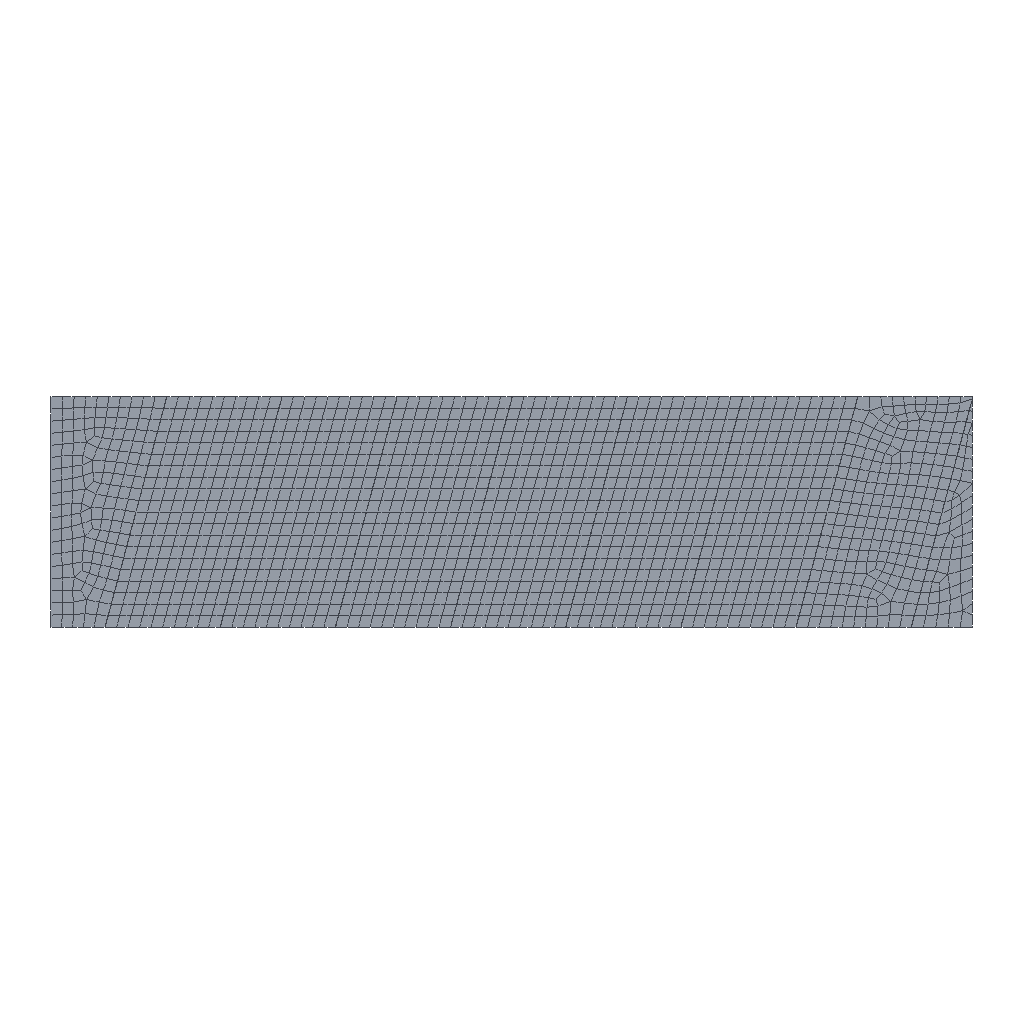Simulation study | abaqus
Set-up summary:
category,name,step,type,value,unit,region
solver,abaqus
solver,version,,,Abaqus/Standard 3DEXPERIENCE R2017x
units,not stated in the deck,,not stated
analysis,deck,,transient,transient
load_step,Step-1,Step-1,transient
load_step,requested,,,1
mesh,nodes,,,2763
mesh,elements,,,2066
element_type,CPS3,,plane,7
element_type,CPS4R,,plane,1643
element_type,COH2D4,,cohesive,416
load,load commands in deck,,count,1
bc,support commands in deck,,count,4
material,COH,,in results
material,CONCRETE,,in results
check,setup vs results,,match,"per instance, exact: element labels, types and connectivity; labels of the nodes the elements use; coordinates of those nodes at SINGLE_PRECISION in 1 of 9 instance(s)"
Abaqus input file, long lists of numbers shortened:
*Heading
** Job name: Job-1 Model name: Model-1
** Generated by: Abaqus/CAE 2017
*Preprint, echo=NO, model=NO, history=NO, contact=NO
**
** PARTS
**
*Part, name=Part-1
*Node
      1,   500.727,           0.
      2,    433.74,        -250.
** (1913 more lines like these left out)
*Element, type=CPS4R
  1,   1,  37, 520,  92
  2,  37,  38, 521, 520
** (1641 more lines like these left out)
*Element, type=CPS3
1201, 1576,  396,  397
1202, 1554, 1581, 1553
** (5 more lines like these left out)
*Nset, nset=Set-1, generate
    1,  1915,     1
*Elset, elset=Set-1, generate
    1,  1650,     1
** Section: concrete
*Solid Section, elset=Set-1, material=concrete
,
*End Part
**
*Part, name=coh
*Node
      1,   58.64,        -250.
      2,   58.74,        -250.
** (104 more lines like these left out)
*Element, type=COH2D4
 1,   1,   2,   5, 106
 2, 106,   5,   6, 105
** (50 more lines like these left out)
*Nset, nset=Set-1, generate
   1,  106,    1
*Elset, elset=Set-1, generate
  1,  52,   1
** Section: Section-2
*Cohesive Section, elset=Set-1, material=coh, response=TRACTION SEPARATION
,
*End Part
**
*Part, name=coh-2
*Node
      1,   183.64,        -250.
      2,   183.74,        -250.
** (104 more lines like these left out)
*Element, type=COH2D4
 1,   1,   2,   5, 106
 2, 106,   5,   6, 105
** (50 more lines like these left out)
*Nset, nset=Set-1, generate
   1,  106,    1
*Elset, elset=Set-1, generate
  1,  52,   1
** Section: Section-2
*Cohesive Section, elset=Set-1, material=coh, response=TRACTION SEPARATION
,
*End Part
**
*Part, name=coh-3
*Node
      1,   308.64,        -250.
      2,    308.74,        -250.
** (104 more lines like these left out)
*Element, type=COH2D4
 1,   1,   2,   5, 106
 2, 106,   5,   6, 105
** (50 more lines like these left out)
*Nset, nset=Set-1, generate
   1,  106,    1
*Elset, elset=Set-1, generate
  1,  52,   1
** Section: Section-2
*Cohesive Section, elset=Set-1, material=coh, response=TRACTION SEPARATION
,
*End Part
**
*Part, name=coh-4
*Node
      1,   433.64,        -250.
      2,    433.74,        -250.
** (104 more lines like these left out)
*Element, type=COH2D4
 1,   1,   2,   5, 106
 2, 106,   5,   6, 105
** (50 more lines like these left out)
*Nset, nset=Set-1, generate
   1,  106,    1
*Elset, elset=Set-1, generate
  1,  52,   1
** Section: Section-2
*Cohesive Section, elset=Set-1, material=coh, response=TRACTION SEPARATION
,
*End Part
**
*Part, name=coh-5
*Node
      1,   558.64,        -250.
      2,    558.74,        -250.
** (104 more lines like these left out)
*Element, type=COH2D4
 1,   1,   2,   5, 106
 2, 106,   5,   6, 105
** (50 more lines like these left out)
*Nset, nset=Set-1, generate
   1,  106,    1
*Elset, elset=Set-1, generate
  1,  52,   1
** Section: Section-2
*Cohesive Section, elset=Set-1, material=coh, response=TRACTION SEPARATION
,
*End Part
**
*Part, name=coh-6
*Node
      1,   683.64,        -250.
      2,    683.74,        -250.
** (104 more lines like these left out)
*Element, type=COH2D4
 1,   1,   2,   5, 106
 2, 106,   5,   6, 105
** (50 more lines like these left out)
*Nset, nset=Set-1, generate
   1,  106,    1
*Elset, elset=Set-1, generate
  1,  52,   1
** Section: Section-2
*Cohesive Section, elset=Set-1, material=coh, response=TRACTION SEPARATION
,
*End Part
**
*Part, name=coh-7
*Node
      1,   808.64,        -250.
      2,    808.74,        -250.
** (104 more lines like these left out)
*Element, type=COH2D4
 1,   1,   2,   5, 106
 2, 106,   5,   6, 105
** (50 more lines like these left out)
*Nset, nset=Set-1, generate
   1,  106,    1
*Elset, elset=Set-1, generate
  1,  52,   1
** Section: Section-2
*Cohesive Section, elset=Set-1, material=coh, response=TRACTION SEPARATION
,
*End Part
**
*Part, name=coh-8
*Node
      1,   933.64,        -250.
      2,    933.74,        -250.
** (104 more lines like these left out)
*Element, type=COH2D4
 1,   1,   2,   5, 106
 2, 106,   5,   6, 105
** (50 more lines like these left out)
*Nset, nset=Set-1, generate
   1,  106,    1
*Elset, elset=Set-1, generate
  1,  52,   1
** Section: Section-2
*Cohesive Section, elset=Set-1, material=coh, response=TRACTION SEPARATION
,
*End Part
**
**
** ASSEMBLY
**
*Assembly, name=Assembly
**
*Instance, name=Part-1-1, part=Part-1
*End Instance
**
*Instance, name=coh-1, part=coh
*End Instance
**
*Instance, name=coh-2-1, part=coh-2
*End Instance
**
*Instance, name=coh-3-1, part=coh-3
*End Instance
**
*Instance, name=coh-4-1, part=coh-4
*End Instance
**
*Instance, name=coh-5-1, part=coh-5
*End Instance
**
*Instance, name=coh-6-1, part=coh-6
*End Instance
**
*Instance, name=coh-7-1, part=coh-7
*End Instance
**
*Instance, name=coh-8-1, part=coh-8
*End Instance
**
*Node
      1,   313.177,           0.,           0.
*Node
      2,   688.177,           0.,           0.
*Nset, nset=Set-2, instance=Part-1-1
  17,  20,  32,  36, 308, 309, 310, 311, 312, 313, 314, 315, 316, 511, 512, 513
 514, 515, 516, 517, 518, 519
*Elset, elset=Set-2, instance=Part-1-1
  801,  821,  841,  861,  881,  901,  921,  941,  961,  981, 1456, 1457, 1460, 1463, 1464, 1467
 1470, 1481, 1513, 1564
*Nset, nset=Set-4, instance=Part-1-1
  25,  26,  27,  28,  30,  31, 392, 393, 394, 395, 396, 397, 398, 399, 400, 401
 402, 403, 404, 405, 406, 407, 408, 409, 410, 411, 412, 413, 442, 443, 444, 445
** (2 more lines like these left out)
*Elset, elset=Set-4, instance=Part-1-1
 1201, 1203, 1204, 1208, 1214, 1217, 1220, 1221, 1222, 1223, 1228, 1230, 1232, 1235, 1237, 1243
 1246, 1248, 1250, 1252, 1253, 1254, 1256, 1266, 1268, 1270, 1271, 1275, 1278, 1288, 1289, 1291
** (1 more lines like these left out)
*Nset, nset=Set-7
 1, 2
*Nset, nset=m_Set-5
 1,
*Nset, nset=m_Set-6
 2,
*Elset, elset=_m_Surf-1_S2, internal, instance=Part-1-1
 1203,
*Elset, elset=_m_Surf-1_S3, internal, instance=Part-1-1
  181,  182,  183,  184,  185,  186,  187,  188,  189,  190,  191,  192,  193,  194,  195,  196
  197,  198,  199,  200,  381,  382,  383,  384,  385,  386,  387,  388,  389,  390,  391,  392
** (8 more lines like these left out)
*Elset, elset=_m_Surf-1_S1, internal, instance=Part-1-1
    1,    2,    3,    4,    5,    6,    7,    8,    9,   10,   11,   12,   13,   14,   15,   16
   17,   18,   19,   20,  201,  202,  203,  204,  205,  206,  207,  208,  209,  210,  211,  212
** (9 more lines like these left out)
*Elset, elset=_m_Surf-1_S4, internal, instance=Part-1-1
 1235,
*Surface, type=ELEMENT, name=m_Surf-1
_m_Surf-1_S2, S2
_m_Surf-1_S3, S3
_m_Surf-1_S4, S4
_m_Surf-1_S1, S1
*Elset, elset=_m_Surf-4_S4, internal, instance=Part-1-1, generate
   1,  181,   20
*Elset, elset=_m_Surf-4_S2, internal, instance=Part-1-1, generate
 420,  600,   20
*Surface, type=ELEMENT, name=m_Surf-4
_m_Surf-4_S4, S4
_m_Surf-4_S2, S2
*Elset, elset=_m_Surf-5_S4, internal, instance=Part-1-1
    1,   21,   41,   61,   81,  101,  121,  141,  161,  181, 1001, 1021, 1041, 1061, 1081, 1101
 1121, 1141, 1161, 1181
*Elset, elset=_m_Surf-5_S2, internal, instance=Part-1-1, generate
 220,  600,   20
*Surface, type=ELEMENT, name=m_Surf-5
_m_Surf-5_S4, S4
_m_Surf-5_S2, S2
*Elset, elset=_m_Surf-6_S2, internal, instance=Part-1-1, generate
 220,  400,   20
*Elset, elset=_m_Surf-6_S4, internal, instance=Part-1-1, generate
 1001,  1181,    20
*Surface, type=ELEMENT, name=m_Surf-6
_m_Surf-6_S2, S2
_m_Surf-6_S4, S4
*Elset, elset=_m_Surf-7_S2, internal, instance=Part-1-1
 1203,
*Elset, elset=_m_Surf-7_S3, internal, instance=Part-1-1
  181,  182,  183,  184,  185,  186,  187,  188,  189,  190,  191,  192,  193,  194,  195,  196
  197,  198,  199,  200,  381,  382,  383,  384,  385,  386,  387,  388,  389,  390,  391,  392
** (8 more lines like these left out)
*Elset, elset=_m_Surf-7_S1, internal, instance=Part-1-1
    1,    2,    3,    4,    5,    6,    7,    8,    9,   10,   11,   12,   13,   14,   15,   16
   17,   18,   19,   20,  201,  202,  203,  204,  205,  206,  207,  208,  209,  210,  211,  212
** (9 more lines like these left out)
*Elset, elset=_m_Surf-7_S4, internal, instance=Part-1-1
 1235,
*Surface, type=ELEMENT, name=m_Surf-7
_m_Surf-7_S2, S2
_m_Surf-7_S3, S3
_m_Surf-7_S4, S4
_m_Surf-7_S1, S1
*Elset, elset=_m_Surf-11_S3, internal, instance=Part-1-1
  981,  982,  983,  984,  985,  986,  987,  988,  989,  990,  991,  992,  993,  994,  995,  996
  997,  998,  999, 1000, 1272, 1274, 1280, 1294, 1295, 1296, 1299, 1303, 1324
*Elset, elset=_m_Surf-11_S1, internal, instance=Part-1-1
 1279, 1281, 1283, 1302, 1310, 1311, 1313, 1316, 1319, 1320, 1345
*Surface, type=ELEMENT, name=m_Surf-11
_m_Surf-11_S3, S3
_m_Surf-11_S1, S1
*Elset, elset=_m_Surf-13_S1, internal, instance=Part-1-1
  801,  802,  803,  804,  805,  806,  807,  808,  809,  810,  811,  812,  813,  814,  815,  816
  817,  818,  819,  820, 1001, 1002, 1003, 1004, 1005, 1006, 1007, 1008, 1009, 1010, 1011, 1012
** (1 more lines like these left out)
*Surface, type=ELEMENT, name=m_Surf-13
_m_Surf-13_S1, S1
*Elset, elset=_m_Surf-15_S3, internal, instance=Part-1-1
  581,  582,  583,  584,  585,  586,  587,  588,  589,  590,  591,  592,  593,  594,  595,  596
  597,  598,  599,  600, 1181, 1182, 1183, 1184, 1185, 1186, 1187, 1188, 1189, 1190, 1191, 1192
** (1 more lines like these left out)
*Surface, type=ELEMENT, name=m_Surf-15
_m_Surf-15_S3, S3
*Elset, elset=_m_Surf-17_S1, internal, instance=Part-1-1
   1,   2,   3,   4,   5,   6,   7,   8,   9,  10,  11,  12,  13,  14,  15,  16
  17,  18,  19,  20, 401, 402, 403, 404, 405, 406, 407, 408, 409, 410, 411, 412
** (1 more lines like these left out)
*Surface, type=ELEMENT, name=m_Surf-17
_m_Surf-17_S1, S1
*Elset, elset=_m_Surf-19_S3, internal, instance=Part-1-1
 181, 182, 183, 184, 185, 186, 187, 188, 189, 190, 191, 192, 193, 194, 195, 196
 197, 198, 199, 200, 381, 382, 383, 384, 385, 386, 387, 388, 389, 390, 391, 392
** (1 more lines like these left out)
*Surface, type=ELEMENT, name=m_Surf-19
_m_Surf-19_S3, S3
*Elset, elset=_m_Surf-21_S1, internal, instance=Part-1-1
 201, 202, 203, 204, 205, 206, 207, 208, 209, 210, 211, 212, 213, 214, 215, 216
 217, 218, 219, 220, 601, 602, 603, 604, 605, 606, 607, 608, 609, 610, 611, 612
** (1 more lines like these left out)
*Surface, type=ELEMENT, name=m_Surf-21
_m_Surf-21_S1, S1
*Elset, elset=_m_Surf-23_S3, internal, instance=Part-1-1
  781,  782,  783,  784,  785,  786,  787,  788,  789,  790,  791,  792,  793,  794,  795,  796
  797,  798,  799,  800, 1424, 1426, 1430, 1434, 1452, 1459, 1461, 1465, 1494, 1508
*Elset, elset=_m_Surf-23_S1, internal, instance=Part-1-1
 1427, 1443, 1444, 1450, 1463, 1479, 1486, 1501, 1509, 1511
*Surface, type=ELEMENT, name=m_Surf-23
_m_Surf-23_S3, S3
_m_Surf-23_S1, S1
*Elset, elset=_m_Surf-25_S2, internal, instance=Part-1-1
 1203,
*Elset, elset=_m_Surf-25_S3, internal, instance=Part-1-1
 1206, 1207, 1210, 1220, 1225, 1234, 1249, 1423, 1425, 1448, 1449, 1469, 1472, 1474, 1480, 1492
 1499,
*Elset, elset=_m_Surf-25_S1, internal, instance=Part-1-1
 1227, 1229, 1231, 1233, 1236, 1238, 1239, 1240, 1241, 1242, 1247, 1431, 1437, 1445, 1453, 1470
 1484, 1485, 1487, 1493, 1500
*Elset, elset=_m_Surf-25_S4, internal, instance=Part-1-1
 1235,
*Surface, type=ELEMENT, name=m_Surf-25
_m_Surf-25_S2, S2
_m_Surf-25_S3, S3
_m_Surf-25_S4, S4
_m_Surf-25_S1, S1
*Elset, elset=_s_Surf-1_S2, internal, instance=coh-1, generate
  1,  52,   1
*Elset, elset=_s_Surf-1_S4, internal, instance=coh-1, generate
  1,  52,   1
*Surface, type=ELEMENT, name=s_Surf-1
_s_Surf-1_S2, S2
_s_Surf-1_S4, S4
*Elset, elset=_s_Surf-3_S2, internal, instance=Part-1-1, generate
 220,  400,   20
*Elset, elset=_s_Surf-3_S4, internal, instance=Part-1-1, generate
 1001,  1181,    20
*Surface, type=ELEMENT, name=s_Surf-3
_s_Surf-3_S2, S2
_s_Surf-3_S4, S4
*Elset, elset=_s_Surf-8_S2, internal, instance=Part-1-1, generate
 220,  400,   20
*Elset, elset=_s_Surf-8_S4, internal, instance=Part-1-1, generate
 1001,  1181,    20
*Surface, type=ELEMENT, name=s_Surf-8
_s_Surf-8_S2, S2
_s_Surf-8_S4, S4
*Elset, elset=_s_Surf-9_S2, internal, instance=Part-1-1, generate
 220,  400,   20
*Elset, elset=_s_Surf-9_S4, internal, instance=Part-1-1, generate
 1001,  1181,    20
*Surface, type=ELEMENT, name=s_Surf-9
_s_Surf-9_S2, S2
_s_Surf-9_S4, S4
*Elset, elset=_s_Surf-10_S2, internal, instance=Part-1-1, generate
 220,  400,   20
*Elset, elset=_s_Surf-10_S4, internal, instance=Part-1-1, generate
 1001,  1181,    20
*Surface, type=ELEMENT, name=s_Surf-10
_s_Surf-10_S2, S2
_s_Surf-10_S4, S4
*Elset, elset=_s_Surf-11_S2, internal, instance=coh-1, generate
  1,  52,   1
*Elset, elset=_s_Surf-11_S4, internal, instance=coh-1, generate
  1,  52,   1
*Surface, type=ELEMENT, name=s_Surf-11
_s_Surf-11_S2, S2
_s_Surf-11_S4, S4
*Elset, elset=_s_Surf-13_S2, internal, instance=coh-2-1, generate
  1,  52,   1
*Elset, elset=_s_Surf-13_S4, internal, instance=coh-2-1, generate
  1,  52,   1
*Surface, type=ELEMENT, name=s_Surf-13
_s_Surf-13_S2, S2
_s_Surf-13_S4, S4
*Elset, elset=_s_Surf-15_S2, internal, instance=coh-3-1, generate
  1,  52,   1
*Elset, elset=_s_Surf-15_S4, internal, instance=coh-3-1, generate
  1,  52,   1
*Surface, type=ELEMENT, name=s_Surf-15
_s_Surf-15_S2, S2
_s_Surf-15_S4, S4
*Elset, elset=_s_Surf-17_S2, internal, instance=coh-4-1, generate
  1,  52,   1
*Elset, elset=_s_Surf-17_S4, internal, instance=coh-4-1, generate
  1,  52,   1
*Surface, type=ELEMENT, name=s_Surf-17
_s_Surf-17_S2, S2
_s_Surf-17_S4, S4
*Elset, elset=_s_Surf-19_S2, internal, instance=coh-5-1, generate
  1,  52,   1
*Elset, elset=_s_Surf-19_S4, internal, instance=coh-5-1, generate
  1,  52,   1
*Surface, type=ELEMENT, name=s_Surf-19
_s_Surf-19_S2, S2
_s_Surf-19_S4, S4
*Elset, elset=_s_Surf-21_S2, internal, instance=coh-6-1, generate
  1,  52,   1
*Elset, elset=_s_Surf-21_S4, internal, instance=coh-6-1, generate
  1,  52,   1
*Surface, type=ELEMENT, name=s_Surf-21
_s_Surf-21_S2, S2
_s_Surf-21_S4, S4
*Elset, elset=_s_Surf-23_S2, internal, instance=coh-7-1, generate
  1,  52,   1
*Elset, elset=_s_Surf-23_S4, internal, instance=coh-7-1, generate
  1,  52,   1
*Surface, type=ELEMENT, name=s_Surf-23
_s_Surf-23_S2, S2
_s_Surf-23_S4, S4
*Elset, elset=_s_Surf-25_S2, internal, instance=coh-8-1, generate
  1,  52,   1
*Elset, elset=_s_Surf-25_S4, internal, instance=coh-8-1, generate
  1,  52,   1
*Surface, type=ELEMENT, name=s_Surf-25
_s_Surf-25_S2, S2
_s_Surf-25_S4, S4
*Elset, elset=_s_Surf-27_S4, internal, instance=Part-1-1, generate
 1001,  1181,    20
*Surface, type=ELEMENT, name=s_Surf-27
_s_Surf-27_S4, S4
*Elset, elset=_s_Surf-28_S2, internal, instance=Part-1-1, generate
 220,  400,   20
*Surface, type=ELEMENT, name=s_Surf-28
_s_Surf-28_S2, S2
** Constraint: Constraint-1
*Tie, name=Constraint-1, adjust=yes
s_Surf-11, m_Surf-11
** Constraint: Constraint-2
*Coupling, constraint name=Constraint-2, ref node=m_Set-5, surface=s_Surf-27
*Kinematic
** Constraint: Constraint-3
*Tie, name=Constraint-3, adjust=yes
s_Surf-13, m_Surf-13
** Constraint: Constraint-4
*Tie, name=Constraint-4, adjust=yes
s_Surf-15, m_Surf-15
** Constraint: Constraint-5
*Tie, name=Constraint-5, adjust=yes
s_Surf-17, m_Surf-17
** Constraint: Constraint-6
*Tie, name=Constraint-6, adjust=yes
s_Surf-19, m_Surf-19
** Constraint: Constraint-7
*Tie, name=Constraint-7, adjust=yes
s_Surf-21, m_Surf-21
** Constraint: Constraint-8
*Tie, name=Constraint-8, adjust=yes
s_Surf-23, m_Surf-23
** Constraint: Constraint-9
*Tie, name=Constraint-9, adjust=yes
s_Surf-25, m_Surf-25
** Constraint: Constraint-10
*Coupling, constraint name=Constraint-10, ref node=m_Set-6, surface=s_Surf-28
*Kinematic
*End Assembly
*Amplitude, name=Amp-1
             0.,              0.,              1.,              1.
**
** MATERIALS
**
*Material, name=coh
*Damage Initiation, criterion=QUADS
 4.5,4.,3.
*Density
 1.8e-09,
*Elastic, type=TRACTION
1000.,1000.,1000.
*Material, name=concrete
*Density
 2.4e-09,
*Elastic
24789., 0.2
*Concrete Damaged Plasticity
30.,   0.1,  1.16, 0.667, 1e-05
*Concrete Compression Hardening
   6.45,      0.
 16.403, 0.00014
 17.684, 0.00019
  18.83, 0.00024
  20.75, 0.00036
 22.222,  0.0005
 23.295, 0.00066
 24.012, 0.00083
 24.411, 0.00102
 24.523, 0.00119
 24.493, 0.00161
 24.388, 0.00202
 24.213, 0.00243
 23.969, 0.00284
 23.661, 0.00325
 23.294, 0.00366
 22.875, 0.00408
 22.286, 0.00461
 21.636, 0.00513
  20.94, 0.00566
  20.21, 0.00619
 19.456, 0.00672
 18.691, 0.00725
 17.158, 0.00831
 15.671, 0.00937
 14.266, 0.01043
 12.965, 0.01148
 11.777, 0.01253
 10.703, 0.01357
  9.737, 0.01461
  8.872, 0.01565
    8.1, 0.01668
   7.41, 0.01771
  6.795, 0.01873
  6.245, 0.01975
  5.313, 0.02179
  4.562, 0.02382
  3.951, 0.02584
   3.45, 0.02786
  3.036, 0.02988
** (4 more lines like these left out)
*Concrete Tension Stiffening
 1.942,      0.
 1.803, 0.00011
 1.674, 0.00021
 1.554, 0.00032
 1.443, 0.00042
 1.339, 0.00052
 1.243, 0.00063
 1.154, 0.00073
 1.072, 0.00083
 0.995, 0.00094
 0.857, 0.00114
 0.739, 0.00135
 0.637, 0.00155
 0.549, 0.00175
 0.473, 0.00196
 0.408, 0.00216
 0.351, 0.00236
 0.303, 0.00256
 0.261, 0.00276
 0.225, 0.00296
 0.194, 0.00317
 0.167, 0.00337
 0.144, 0.00357
 0.124, 0.00377
 0.107, 0.00397
*Concrete Compression Damage
     0.,      0.
 0.0909, 0.00014
 0.1101, 0.00019
 0.1289, 0.00024
 0.1653, 0.00036
 0.2004,  0.0005
 0.2342, 0.00066
 0.2671, 0.00083
  0.299, 0.00102
  0.327, 0.00119
 0.3843, 0.00161
 0.4282, 0.00202
 0.4649, 0.00243
 0.4965, 0.00284
 0.5243, 0.00325
 0.5491, 0.00366
 0.5715, 0.00408
 0.5968, 0.00461
 0.6197, 0.00513
 0.6407, 0.00566
 0.6599, 0.00619
 0.6777, 0.00672
 0.6942, 0.00725
 0.7239, 0.00831
 0.7498, 0.00937
 0.7725, 0.01043
 0.7925, 0.01148
 0.8101, 0.01253
 0.8256, 0.01357
 0.8394, 0.01461
 0.8516, 0.01565
 0.8625, 0.01668
 0.8723, 0.01771
  0.881, 0.01873
 0.8889, 0.01975
 0.9024, 0.02179
 0.9135, 0.02382
 0.9227, 0.02584
 0.9305, 0.02786
  0.937, 0.02988
** (15 more lines like these left out)
*Concrete Tension Damage
    0.,      0.
 0.361, 0.00011
 0.507, 0.00021
 0.593, 0.00032
 0.651, 0.00042
 0.694, 0.00052
 0.728, 0.00063
 0.755, 0.00073
 0.778, 0.00083
 0.797, 0.00094
 0.829, 0.00114
 0.853, 0.00135
 0.872, 0.00155
 0.888, 0.00175
 0.902, 0.00196
 0.913, 0.00216
 0.923, 0.00236
 0.931, 0.00256
 0.938, 0.00276
 0.945, 0.00296
  0.95, 0.00317
 0.955, 0.00337
  0.96, 0.00357
 0.964, 0.00377
 0.967, 0.00397
**
** INTERACTION PROPERTIES
**
*Surface Interaction, name=IntProp-1
1.,
*Friction, slip tolerance=0.005
 0.3,
*Surface Behavior, pressure-overclosure=HARD
**
** INTERACTIONS
**
** Interaction: Int-1
*Contact
*Contact Inclusions, ALL EXTERIOR
*Contact Property Assignment
 ,  , IntProp-1
** ----------------------------------------------------------------
**
** STEP: Step-1
**
*Step, name=Step-1, nlgeom=YES, inc=1000
*Dynamic
0.001,1.,1e-05
**
** BOUNDARY CONDITIONS
**
** Name: BC-1 Type: 对称/反对称/完全固定
*Boundary
Set-4, ENCASTRE
** Name: BC-2 Type: 位移/转角
*Boundary
Set-7, 1, 1
Set-7, 2, 2, -20.
Set-7, 6, 6
**
** CONTROLS
**
*Controls, reset
*Controls, parameters=time incrementation
, , , , , , , 20, , ,
**
** OUTPUT REQUESTS
**
*Restart, write, frequency=0
**
** FIELD OUTPUT: F-Output-1
**
*Output, field, frequency=1
*Node Output
CF, RF, U, V
*Element Output, directions=YES
DAMAGEC, DAMAGET, E, LE, MISES, PE, PEEQ, PEMAG, S, SDEG
*Contact Output
CDISP, CSDMG, CSTRESS
**
** HISTORY OUTPUT: H-Output-1
**
*Output, history, frequency=1
*Node Output, nset=Set-7
RF1, RF2, U1, U2
*End Step
Results summary:
result,step,,partial,increments=13 time=0.006428/1.0
result,analysis,,,transient
result,last_loadstep,,,1
result,primary field,,,U
result,reaction total,,FX,-2161220308244030000000000,model units
result,reaction total,,FY,14989867906747812000000000000000,model units
result,reaction total,,FZ,0.0,model units